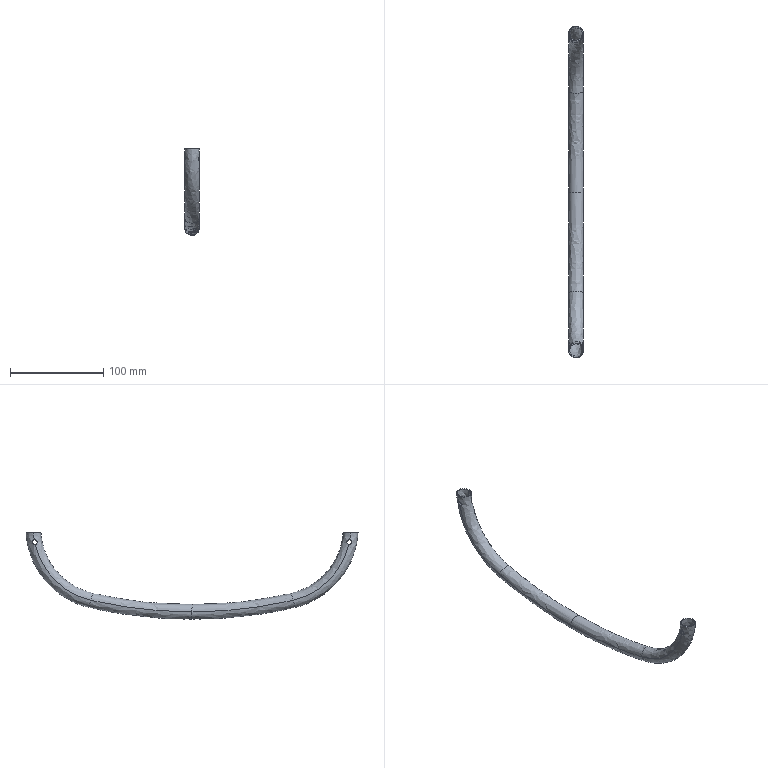Part | SolidWorks | features BaseBody 1 | 1 solid | 26 faces | box 16 x 356.5 x 92.983 mm | volume 16054 mm3 | spline 16 | cylinder 8 | plane 2 | commonest cylinder face diameters 5.2 x8